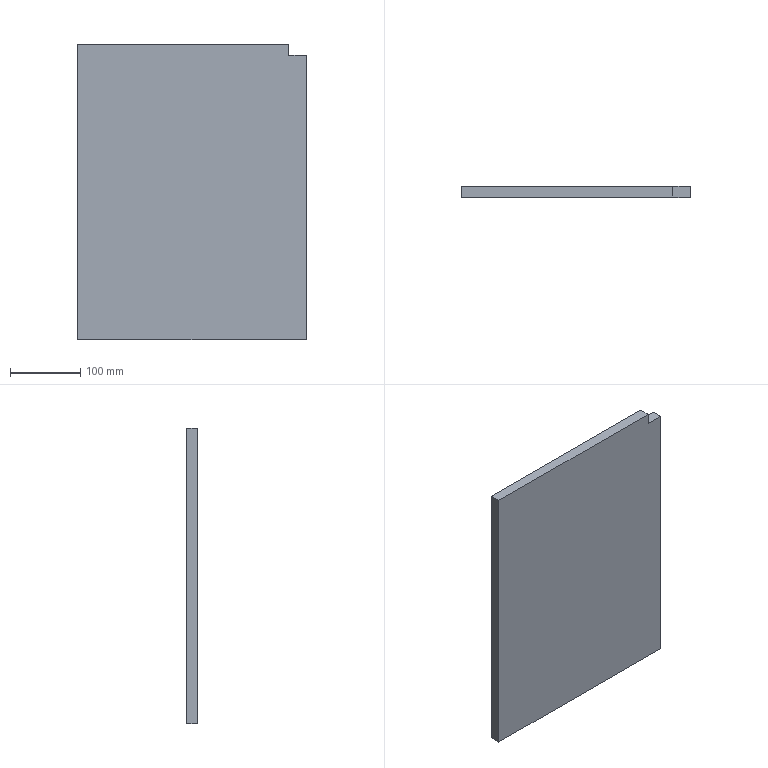Part | SolidWorks | features Extrusion 1 | 1 solid | 8 faces | box 325 x 15 x 420 mm | volume 2041500 mm3 | plane 8
STEP:
#1=CARTESIAN_POINT('',(300.,0.,404.));
#2=VERTEX_POINT('',#1);
#3=CARTESIAN_POINT('',(300.,0.,420.));
#4=VERTEX_POINT('',#3);
#5=CARTESIAN_POINT('',(300.,0.,404.));
#6=DIRECTION('',(0.,0.,1.));
#7=VECTOR('',#6,1000.);
#8=LINE('',#5,#7);
#9=EDGE_CURVE('',#2,#4,#8,.T.);
#10=ORIENTED_EDGE('',*,*,#9,.F.);
#11=CARTESIAN_POINT('',(300.,15.,404.));
#12=VERTEX_POINT('',#11);
#13=CARTESIAN_POINT('',(300.,15.,404.));
#14=DIRECTION('',(0.,-1.,0.));
#15=VECTOR('',#14,1000.);
#16=LINE('',#13,#15);
#17=EDGE_CURVE('',#12,#2,#16,.T.);
#18=ORIENTED_EDGE('',*,*,#17,.F.);
#19=CARTESIAN_POINT('',(300.,15.,420.));
#20=VERTEX_POINT('',#19);
#21=CARTESIAN_POINT('',(300.,15.,404.));
#22=DIRECTION('',(0.,0.,1.));
#23=VECTOR('',#22,1000.);
#24=LINE('',#21,#23);
#25=EDGE_CURVE('',#12,#20,#24,.T.);
#26=ORIENTED_EDGE('',*,*,#25,.T.);
#27=CARTESIAN_POINT('',(300.,15.,420.));
#28=DIRECTION('',(0.,-1.,0.));
#29=VECTOR('',#28,1000.);
#30=LINE('',#27,#29);
#31=EDGE_CURVE('',#20,#4,#30,.T.);
#32=ORIENTED_EDGE('',*,*,#31,.T.);
#33=EDGE_LOOP('',(#10,#18,#26,#32));
#34=FACE_OUTER_BOUND('',#33,.T.);
#35=CARTESIAN_POINT('',(300.,15.,404.));
#36=DIRECTION('',(1.,0.,0.));
#37=DIRECTION('',(0.,0.,-1.));
#38=AXIS2_PLACEMENT_3D('',#35,#36,#37);
#39=PLANE('',#38);
#40=ADVANCED_FACE('',(#34),#39,.T.);
#41=CARTESIAN_POINT('',(325.,0.,404.));
#42=VERTEX_POINT('',#41);
#43=CARTESIAN_POINT('',(325.,0.,404.));
#44=DIRECTION('',(-1.,0.,0.));
#45=VECTOR('',#44,1000.);
#46=LINE('',#43,#45);
#47=EDGE_CURVE('',#42,#2,#46,.T.);
#48=ORIENTED_EDGE('',*,*,#47,.F.);
#49=CARTESIAN_POINT('',(325.,15.,404.));
#50=VERTEX_POINT('',#49);
#51=CARTESIAN_POINT('',(325.,15.,404.));
#52=DIRECTION('',(0.,-1.,0.));
#53=VECTOR('',#52,1000.);
#54=LINE('',#51,#53);
#55=EDGE_CURVE('',#50,#42,#54,.T.);
#56=ORIENTED_EDGE('',*,*,#55,.F.);
#57=CARTESIAN_POINT('',(325.,15.,404.));
#58=DIRECTION('',(-1.,0.,0.));
#59=VECTOR('',#58,1000.);
#60=LINE('',#57,#59);
#61=EDGE_CURVE('',#50,#12,#60,.T.);
#62=ORIENTED_EDGE('',*,*,#61,.T.);
#63=ORIENTED_EDGE('',*,*,#17,.T.);
#64=EDGE_LOOP('',(#48,#56,#62,#63));
#65=FACE_OUTER_BOUND('',#64,.T.);
#66=CARTESIAN_POINT('',(325.,15.,404.));
#67=DIRECTION('',(0.,0.,1.));
#68=DIRECTION('',(1.,0.,0.));
#69=AXIS2_PLACEMENT_3D('',#66,#67,#68);
#70=PLANE('',#69);
#71=ADVANCED_FACE('',(#65),#70,.T.);
#72=CARTESIAN_POINT('',(325.,0.,0.));
#73=VERTEX_POINT('',#72);
#74=CARTESIAN_POINT('',(325.,0.,0.));
#75=DIRECTION('',(0.,0.,1.));
#76=VECTOR('',#75,1000.);
#77=LINE('',#74,#76);
#78=EDGE_CURVE('',#73,#42,#77,.T.);
#79=ORIENTED_EDGE('',*,*,#78,.F.);
#80=CARTESIAN_POINT('',(325.,15.,0.));
#81=VERTEX_POINT('',#80);
#82=CARTESIAN_POINT('',(325.,15.,0.));
#83=DIRECTION('',(0.,-1.,0.));
#84=VECTOR('',#83,1000.);
#85=LINE('',#82,#84);
#86=EDGE_CURVE('',#81,#73,#85,.T.);
#87=ORIENTED_EDGE('',*,*,#86,.F.);
#88=CARTESIAN_POINT('',(325.,15.,0.));
#89=DIRECTION('',(0.,0.,1.));
#90=VECTOR('',#89,1000.);
#91=LINE('',#88,#90);
#92=EDGE_CURVE('',#81,#50,#91,.T.);
#93=ORIENTED_EDGE('',*,*,#92,.T.);
#94=ORIENTED_EDGE('',*,*,#55,.T.);
#95=EDGE_LOOP('',(#79,#87,#93,#94));
#96=FACE_OUTER_BOUND('',#95,.T.);
#97=CARTESIAN_POINT('',(325.,15.,0.));
#98=DIRECTION('',(1.,0.,0.));
#99=DIRECTION('',(0.,0.,-1.));
#100=AXIS2_PLACEMENT_3D('',#97,#98,#99);
#101=PLANE('',#100);
#102=ADVANCED_FACE('',(#96),#101,.T.);
#103=CARTESIAN_POINT('',(0.,0.,0.));
#104=VERTEX_POINT('',#103);
#105=CARTESIAN_POINT('',(0.,0.,0.));
#106=DIRECTION('',(1.,0.,0.));
#107=VECTOR('',#106,1000.);
#108=LINE('',#105,#107);
#109=EDGE_CURVE('',#104,#73,#108,.T.);
#110=ORIENTED_EDGE('',*,*,#109,.F.);
#111=CARTESIAN_POINT('',(0.,15.,0.));
#112=VERTEX_POINT('',#111);
#113=CARTESIAN_POINT('',(0.,15.,0.));
#114=DIRECTION('',(0.,-1.,0.));
#115=VECTOR('',#114,1000.);
#116=LINE('',#113,#115);
#117=EDGE_CURVE('',#112,#104,#116,.T.);
#118=ORIENTED_EDGE('',*,*,#117,.F.);
#119=CARTESIAN_POINT('',(0.,15.,0.));
#120=DIRECTION('',(1.,0.,0.));
#121=VECTOR('',#120,1000.);
#122=LINE('',#119,#121);
#123=EDGE_CURVE('',#112,#81,#122,.T.);
#124=ORIENTED_EDGE('',*,*,#123,.T.);
#125=ORIENTED_EDGE('',*,*,#86,.T.);
#126=EDGE_LOOP('',(#110,#118,#124,#125));
#127=FACE_OUTER_BOUND('',#126,.T.);
#128=CARTESIAN_POINT('',(0.,15.,0.));
#129=DIRECTION('',(0.,0.,-1.));
#130=DIRECTION('',(-1.,0.,0.));
#131=AXIS2_PLACEMENT_3D('',#128,#129,#130);
#132=PLANE('',#131);
#133=ADVANCED_FACE('',(#127),#132,.T.);
#134=CARTESIAN_POINT('',(0.,0.,420.));
#135=VERTEX_POINT('',#134);
#136=CARTESIAN_POINT('',(0.,0.,420.));
#137=DIRECTION('',(0.,0.,-1.));
#138=VECTOR('',#137,1000.);
#139=LINE('',#136,#138);
#140=EDGE_CURVE('',#135,#104,#139,.T.);
#141=ORIENTED_EDGE('',*,*,#140,.F.);
#142=CARTESIAN_POINT('',(0.,15.,420.));
#143=VERTEX_POINT('',#142);
#144=CARTESIAN_POINT('',(0.,15.,420.));
#145=DIRECTION('',(0.,-1.,0.));
#146=VECTOR('',#145,1000.);
#147=LINE('',#144,#146);
#148=EDGE_CURVE('',#143,#135,#147,.T.);
#149=ORIENTED_EDGE('',*,*,#148,.F.);
#150=CARTESIAN_POINT('',(0.,15.,420.));
#151=DIRECTION('',(0.,0.,-1.));
#152=VECTOR('',#151,1000.);
#153=LINE('',#150,#152);
#154=EDGE_CURVE('',#143,#112,#153,.T.);
#155=ORIENTED_EDGE('',*,*,#154,.T.);
#156=ORIENTED_EDGE('',*,*,#117,.T.);
#157=EDGE_LOOP('',(#141,#149,#155,#156));
#158=FACE_OUTER_BOUND('',#157,.T.);
#159=CARTESIAN_POINT('',(0.,15.,420.));
#160=DIRECTION('',(-1.,0.,0.));
#161=DIRECTION('',(0.,0.,1.));
#162=AXIS2_PLACEMENT_3D('',#159,#160,#161);
#163=PLANE('',#162);
#164=ADVANCED_FACE('',(#158),#163,.T.);
#165=CARTESIAN_POINT('',(300.,0.,420.));
#166=DIRECTION('',(-1.,0.,0.));
#167=VECTOR('',#166,1000.);
#168=LINE('',#165,#167);
#169=EDGE_CURVE('',#4,#135,#168,.T.);
#170=ORIENTED_EDGE('',*,*,#169,.F.);
#171=ORIENTED_EDGE('',*,*,#31,.F.);
#172=CARTESIAN_POINT('',(300.,15.,420.));
#173=DIRECTION('',(-1.,0.,0.));
#174=VECTOR('',#173,1000.);
#175=LINE('',#172,#174);
#176=EDGE_CURVE('',#20,#143,#175,.T.);
#177=ORIENTED_EDGE('',*,*,#176,.T.);
#178=ORIENTED_EDGE('',*,*,#148,.T.);
#179=EDGE_LOOP('',(#170,#171,#177,#178));
#180=FACE_OUTER_BOUND('',#179,.T.);
#181=CARTESIAN_POINT('',(300.,15.,420.));
#182=DIRECTION('',(0.,0.,1.));
#183=DIRECTION('',(1.,0.,0.));
#184=AXIS2_PLACEMENT_3D('',#181,#182,#183);
#185=PLANE('',#184);
#186=ADVANCED_FACE('',(#180),#185,.T.);
#187=ORIENTED_EDGE('',*,*,#25,.F.);
#188=ORIENTED_EDGE('',*,*,#61,.F.);
#189=ORIENTED_EDGE('',*,*,#92,.F.);
#190=ORIENTED_EDGE('',*,*,#123,.F.);
#191=ORIENTED_EDGE('',*,*,#154,.F.);
#192=ORIENTED_EDGE('',*,*,#176,.F.);
#193=EDGE_LOOP('',(#187,#188,#189,#190,#191,#192));
#194=FACE_OUTER_BOUND('',#193,.T.);
#195=CARTESIAN_POINT('',(0.,15.,0.));
#196=DIRECTION('',(0.,-1.,0.));
#197=DIRECTION('',(0.,0.,-1.));
#198=AXIS2_PLACEMENT_3D('',#195,#196,#197);
#199=PLANE('',#198);
#200=ADVANCED_FACE('',(#194),#199,.F.);
#201=ORIENTED_EDGE('',*,*,#9,.T.);
#202=ORIENTED_EDGE('',*,*,#169,.T.);
#203=ORIENTED_EDGE('',*,*,#140,.T.);
#204=ORIENTED_EDGE('',*,*,#109,.T.);
#205=ORIENTED_EDGE('',*,*,#78,.T.);
#206=ORIENTED_EDGE('',*,*,#47,.T.);
#207=EDGE_LOOP('',(#201,#202,#203,#204,#205,#206));
#208=FACE_OUTER_BOUND('',#207,.T.);
#209=CARTESIAN_POINT('',(0.,0.,0.));
#210=DIRECTION('',(0.,-1.,0.));
#211=DIRECTION('',(0.,0.,-1.));
#212=AXIS2_PLACEMENT_3D('',#209,#210,#211);
#213=PLANE('',#212);
#214=ADVANCED_FACE('',(#208),#213,.T.);
#215=CLOSED_SHELL('',(#40,#71,#102,#133,#164,#186,#200,#214));
#216=MANIFOLD_SOLID_BREP('',#215);
#217=CARTESIAN_POINT('',(0.,0.,0.));
#218=DIRECTION('',(0.,0.,1.));
#219=DIRECTION('',(1.,0.,0.));
#220=AXIS2_PLACEMENT_3D('',#217,#218,#219);
#221=(LENGTH_UNIT()NAMED_UNIT(*)SI_UNIT(.MILLI.,.METRE.));
#222=UNCERTAINTY_MEASURE_WITH_UNIT(LENGTH_MEASURE(0.00001),#221,'','');
#223=(NAMED_UNIT(*)PLANE_ANGLE_UNIT()SI_UNIT($,.RADIAN.));
#224=(NAMED_UNIT(*)SI_UNIT($,.STERADIAN.)SOLID_ANGLE_UNIT());
#225=(GEOMETRIC_REPRESENTATION_CONTEXT(3)GLOBAL_UNCERTAINTY_ASSIGNED_CONTEXT((#222))GLOBAL_UNIT_ASSIGNED_CONTEXT((#221,#223,#224))REPRESENTATION_CONTEXT('',''));
#226=ADVANCED_BREP_SHAPE_REPRESENTATION('',(#216,#220),#225);